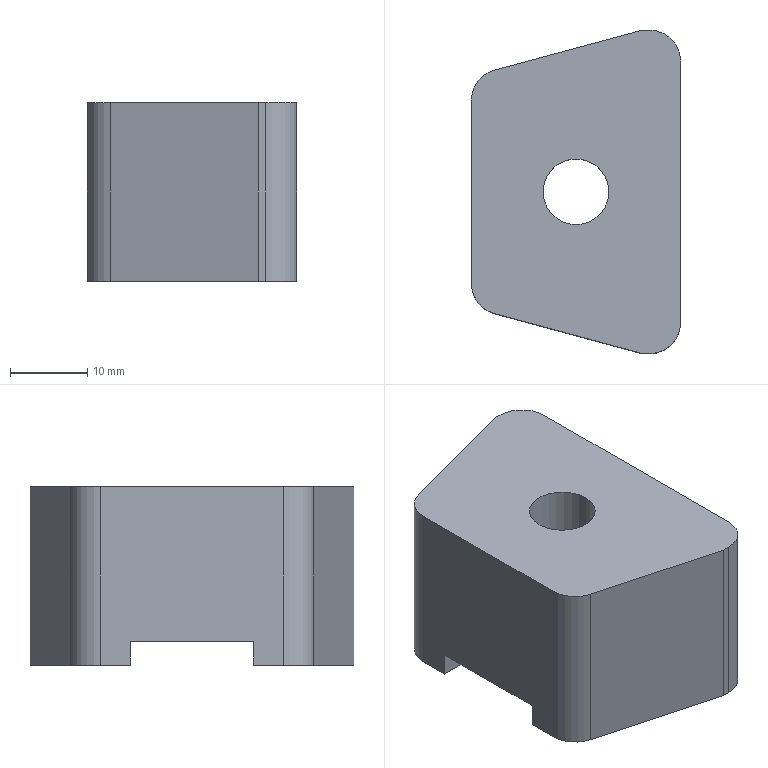Part | NX | features solid 2 | 1 solid | 19 faces | box 27 x 41.761 x 23 mm | volume 19258 mm3 | plane 13 | cylinder 6 | commonest cylinder face diameters 8 x4 8.5 x1 14 x1
STEP:
#1=CARTESIAN_POINT('',(636.324,0.,20.));
#2=VERTEX_POINT('',#1);
#3=CARTESIAN_POINT('',(632.074,0.,20.));
#4=DIRECTION('',(0.,0.,1.));
#5=DIRECTION('',(1.,0.,0.));
#6=AXIS2_PLACEMENT_3D('',#3,#4,#5);
#7=CIRCLE('',#6,4.25);
#8=EDGE_CURVE('',#2,#2,#7,.T.);
#9=ORIENTED_EDGE('',*,*,#8,.F.);
#10=EDGE_LOOP('',(#9));
#11=FACE_BOUND('',#10,.T.);
#12=CARTESIAN_POINT('',(640.659,-20.88,20.));
#13=VERTEX_POINT('',#12);
#14=CARTESIAN_POINT('',(641.574,-20.88,20.));
#15=VERTEX_POINT('',#14);
#16=CARTESIAN_POINT('',(704.285,-20.88,20.));
#17=DIRECTION('',(1.,0.,0.));
#18=VECTOR('',#17,1000.);
#19=LINE('',#16,#18);
#20=EDGE_CURVE('',#13,#15,#19,.T.);
#21=ORIENTED_EDGE('',*,*,#20,.T.);
#22=CARTESIAN_POINT('',(645.574,-16.88,20.));
#23=VERTEX_POINT('',#22);
#24=CARTESIAN_POINT('',(641.574,-16.88,20.));
#25=DIRECTION('',(0.,0.,1.));
#26=DIRECTION('',(1.,0.,0.));
#27=AXIS2_PLACEMENT_3D('',#24,#25,#26);
#28=CIRCLE('',#27,4.);
#29=EDGE_CURVE('',#15,#23,#28,.T.);
#30=ORIENTED_EDGE('',*,*,#29,.T.);
#31=CARTESIAN_POINT('',(645.574,16.88,20.));
#32=VERTEX_POINT('',#31);
#33=CARTESIAN_POINT('',(645.574,-11.19,20.));
#34=DIRECTION('',(0.,-1.,0.));
#35=VECTOR('',#34,1000.);
#36=LINE('',#33,#35);
#37=EDGE_CURVE('',#32,#23,#36,.T.);
#38=ORIENTED_EDGE('',*,*,#37,.F.);
#39=CARTESIAN_POINT('',(641.574,20.88,20.));
#40=VERTEX_POINT('',#39);
#41=CARTESIAN_POINT('',(641.574,16.88,20.));
#42=DIRECTION('',(0.,0.,1.));
#43=DIRECTION('',(1.,0.,0.));
#44=AXIS2_PLACEMENT_3D('',#41,#42,#43);
#45=CIRCLE('',#44,4.);
#46=EDGE_CURVE('',#32,#40,#45,.T.);
#47=ORIENTED_EDGE('',*,*,#46,.T.);
#48=CARTESIAN_POINT('',(640.659,20.88,20.));
#49=VERTEX_POINT('',#48);
#50=CARTESIAN_POINT('',(704.285,20.88,20.));
#51=DIRECTION('',(-1.,0.,0.));
#52=VECTOR('',#51,1000.);
#53=LINE('',#50,#52);
#54=EDGE_CURVE('',#40,#49,#53,.T.);
#55=ORIENTED_EDGE('',*,*,#54,.T.);
#56=CARTESIAN_POINT('',(621.53,15.711,20.));
#57=VERTEX_POINT('',#56);
#58=CARTESIAN_POINT('',(666.85,27.959,20.));
#59=DIRECTION('',(0.9654,0.2609,0.));
#60=VECTOR('',#59,1000.);
#61=LINE('',#58,#60);
#62=EDGE_CURVE('',#49,#57,#61,.F.);
#63=ORIENTED_EDGE('',*,*,#62,.T.);
#64=CARTESIAN_POINT('',(618.574,11.849,20.));
#65=VERTEX_POINT('',#64);
#66=CARTESIAN_POINT('',(622.574,11.849,20.));
#67=DIRECTION('',(0.,0.,1.));
#68=DIRECTION('',(1.,0.,0.));
#69=AXIS2_PLACEMENT_3D('',#66,#67,#68);
#70=CIRCLE('',#69,4.);
#71=EDGE_CURVE('',#57,#65,#70,.T.);
#72=ORIENTED_EDGE('',*,*,#71,.T.);
#73=CARTESIAN_POINT('',(618.574,-11.849,20.));
#74=VERTEX_POINT('',#73);
#75=CARTESIAN_POINT('',(618.574,-7.,20.));
#76=DIRECTION('',(0.,1.,0.));
#77=VECTOR('',#76,1000.);
#78=LINE('',#75,#77);
#79=EDGE_CURVE('',#74,#65,#78,.T.);
#80=ORIENTED_EDGE('',*,*,#79,.F.);
#81=CARTESIAN_POINT('',(621.53,-15.711,20.));
#82=VERTEX_POINT('',#81);
#83=CARTESIAN_POINT('',(622.574,-11.849,20.));
#84=DIRECTION('',(0.,0.,1.));
#85=DIRECTION('',(1.,0.,0.));
#86=AXIS2_PLACEMENT_3D('',#83,#84,#85);
#87=CIRCLE('',#86,4.);
#88=EDGE_CURVE('',#74,#82,#87,.T.);
#89=ORIENTED_EDGE('',*,*,#88,.T.);
#90=CARTESIAN_POINT('',(722.538,-43.01,20.));
#91=DIRECTION('',(-0.9654,0.2609,0.));
#92=VECTOR('',#91,1000.);
#93=LINE('',#90,#92);
#94=EDGE_CURVE('',#82,#13,#93,.F.);
#95=ORIENTED_EDGE('',*,*,#94,.T.);
#96=EDGE_LOOP('',(#21,#30,#38,#47,#55,#63,#72,#80,#89,#95));
#97=FACE_BOUND('',#96,.T.);
#98=CARTESIAN_POINT('',(704.285,-110.548,20.));
#99=DIRECTION('',(0.,0.,1.));
#100=DIRECTION('',(1.,0.,0.));
#101=AXIS2_PLACEMENT_3D('',#98,#99,#100);
#102=PLANE('',#101);
#103=ADVANCED_FACE('',(#11,#97),#102,.T.);
#104=CARTESIAN_POINT('',(645.574,-8.,0.));
#105=VERTEX_POINT('',#104);
#106=CARTESIAN_POINT('',(618.574,-8.,0.));
#107=VERTEX_POINT('',#106);
#108=CARTESIAN_POINT('',(630.85,-8.,0.));
#109=DIRECTION('',(-1.,0.,0.));
#110=VECTOR('',#109,1000.);
#111=LINE('',#108,#110);
#112=EDGE_CURVE('',#105,#107,#111,.T.);
#113=ORIENTED_EDGE('',*,*,#112,.F.);
#114=CARTESIAN_POINT('',(645.574,-8.,-3.));
#115=VERTEX_POINT('',#114);
#116=CARTESIAN_POINT('',(645.574,-8.,-5.));
#117=DIRECTION('',(0.,0.,1.));
#118=VECTOR('',#117,1000.);
#119=LINE('',#116,#118);
#120=EDGE_CURVE('',#115,#105,#119,.T.);
#121=ORIENTED_EDGE('',*,*,#120,.F.);
#122=CARTESIAN_POINT('',(618.574,-8.,-3.));
#123=VERTEX_POINT('',#122);
#124=CARTESIAN_POINT('',(268.879,-8.,-3.));
#125=DIRECTION('',(-1.,0.,0.));
#126=VECTOR('',#125,1000.);
#127=LINE('',#124,#126);
#128=EDGE_CURVE('',#123,#115,#127,.F.);
#129=ORIENTED_EDGE('',*,*,#128,.F.);
#130=CARTESIAN_POINT('',(618.574,-8.,-5.));
#131=DIRECTION('',(0.,0.,1.));
#132=VECTOR('',#131,1000.);
#133=LINE('',#130,#132);
#134=EDGE_CURVE('',#123,#107,#133,.T.);
#135=ORIENTED_EDGE('',*,*,#134,.T.);
#136=EDGE_LOOP('',(#113,#121,#129,#135));
#137=FACE_BOUND('',#136,.T.);
#138=CARTESIAN_POINT('',(630.85,-8.,-5.));
#139=DIRECTION('',(0.,1.,0.));
#140=DIRECTION('',(0.,0.,-1.));
#141=AXIS2_PLACEMENT_3D('',#138,#139,#140);
#142=PLANE('',#141);
#143=ADVANCED_FACE('',(#137),#142,.T.);
#144=CARTESIAN_POINT('',(645.574,-16.88,-3.));
#145=VERTEX_POINT('',#144);
#146=CARTESIAN_POINT('',(645.574,0.,-3.));
#147=DIRECTION('',(0.,1.,0.));
#148=VECTOR('',#147,1000.);
#149=LINE('',#146,#148);
#150=EDGE_CURVE('',#115,#145,#149,.F.);
#151=ORIENTED_EDGE('',*,*,#150,.T.);
#152=CARTESIAN_POINT('',(641.574,-20.88,-3.));
#153=VERTEX_POINT('',#152);
#154=CARTESIAN_POINT('',(641.574,-16.88,-3.));
#155=DIRECTION('',(0.,0.,1.));
#156=DIRECTION('',(1.,0.,0.));
#157=AXIS2_PLACEMENT_3D('',#154,#155,#156);
#158=CIRCLE('',#157,4.);
#159=EDGE_CURVE('',#145,#153,#158,.F.);
#160=ORIENTED_EDGE('',*,*,#159,.T.);
#161=CARTESIAN_POINT('',(640.659,-20.88,-3.));
#162=VERTEX_POINT('',#161);
#163=CARTESIAN_POINT('',(268.879,-20.88,-3.));
#164=DIRECTION('',(1.,0.,0.));
#165=VECTOR('',#164,1000.);
#166=LINE('',#163,#165);
#167=EDGE_CURVE('',#153,#162,#166,.F.);
#168=ORIENTED_EDGE('',*,*,#167,.T.);
#169=CARTESIAN_POINT('',(621.53,-15.711,-3.));
#170=VERTEX_POINT('',#169);
#171=CARTESIAN_POINT('',(637.087,-19.915,-3.));
#172=DIRECTION('',(0.9654,-0.2609,0.));
#173=VECTOR('',#172,1000.);
#174=LINE('',#171,#173);
#175=EDGE_CURVE('',#170,#162,#174,.T.);
#176=ORIENTED_EDGE('',*,*,#175,.F.);
#177=CARTESIAN_POINT('',(618.574,-11.849,-3.));
#178=VERTEX_POINT('',#177);
#179=CARTESIAN_POINT('',(622.574,-11.849,-3.));
#180=DIRECTION('',(0.,0.,1.));
#181=DIRECTION('',(1.,0.,0.));
#182=AXIS2_PLACEMENT_3D('',#179,#180,#181);
#183=CIRCLE('',#182,4.);
#184=EDGE_CURVE('',#170,#178,#183,.F.);
#185=ORIENTED_EDGE('',*,*,#184,.T.);
#186=CARTESIAN_POINT('',(618.574,0.,-3.));
#187=DIRECTION('',(0.,-1.,0.));
#188=VECTOR('',#187,1000.);
#189=LINE('',#186,#188);
#190=EDGE_CURVE('',#178,#123,#189,.F.);
#191=ORIENTED_EDGE('',*,*,#190,.T.);
#192=ORIENTED_EDGE('',*,*,#128,.T.);
#193=EDGE_LOOP('',(#151,#160,#168,#176,#185,#191,#192));
#194=FACE_BOUND('',#193,.T.);
#195=CARTESIAN_POINT('',(268.879,0.,-3.));
#196=DIRECTION('',(0.,0.,1.));
#197=DIRECTION('',(1.,0.,0.));
#198=AXIS2_PLACEMENT_3D('',#195,#196,#197);
#199=PLANE('',#198);
#200=ADVANCED_FACE('',(#194),#199,.F.);
#201=ORIENTED_EDGE('',*,*,#94,.F.);
#202=CARTESIAN_POINT('',(621.53,-15.711,-5.));
#203=DIRECTION('',(0.,0.,-1.));
#204=VECTOR('',#203,1000.);
#205=LINE('',#202,#204);
#206=EDGE_CURVE('',#82,#170,#205,.T.);
#207=ORIENTED_EDGE('',*,*,#206,.T.);
#208=ORIENTED_EDGE('',*,*,#175,.T.);
#209=CARTESIAN_POINT('',(640.659,-20.88,-5.));
#210=DIRECTION('',(0.,0.,-1.));
#211=VECTOR('',#210,1000.);
#212=LINE('',#209,#211);
#213=EDGE_CURVE('',#162,#13,#212,.F.);
#214=ORIENTED_EDGE('',*,*,#213,.T.);
#215=EDGE_LOOP('',(#201,#207,#208,#214));
#216=FACE_BOUND('',#215,.T.);
#217=CARTESIAN_POINT('',(637.087,-19.915,-5.));
#218=DIRECTION('',(0.2609,0.9654,0.));
#219=DIRECTION('',(0.,0.,1.));
#220=AXIS2_PLACEMENT_3D('',#217,#218,#219);
#221=PLANE('',#220);
#222=ADVANCED_FACE('',(#216),#221,.F.);
#223=ORIENTED_EDGE('',*,*,#167,.F.);
#224=CARTESIAN_POINT('',(641.574,-20.88,-5.));
#225=DIRECTION('',(0.,0.,1.));
#226=VECTOR('',#225,1000.);
#227=LINE('',#224,#226);
#228=EDGE_CURVE('',#153,#15,#227,.T.);
#229=ORIENTED_EDGE('',*,*,#228,.T.);
#230=ORIENTED_EDGE('',*,*,#20,.F.);
#231=ORIENTED_EDGE('',*,*,#213,.F.);
#232=EDGE_LOOP('',(#223,#229,#230,#231));
#233=FACE_BOUND('',#232,.T.);
#234=CARTESIAN_POINT('',(630.85,-20.88,-5.));
#235=DIRECTION('',(0.,-1.,0.));
#236=DIRECTION('',(0.,0.,1.));
#237=AXIS2_PLACEMENT_3D('',#234,#235,#236);
#238=PLANE('',#237);
#239=ADVANCED_FACE('',(#233),#238,.T.);
#240=ORIENTED_EDGE('',*,*,#37,.T.);
#241=CARTESIAN_POINT('',(645.574,-16.88,-5.));
#242=DIRECTION('',(0.,0.,1.));
#243=VECTOR('',#242,1000.);
#244=LINE('',#241,#243);
#245=EDGE_CURVE('',#23,#145,#244,.F.);
#246=ORIENTED_EDGE('',*,*,#245,.T.);
#247=ORIENTED_EDGE('',*,*,#150,.F.);
#248=ORIENTED_EDGE('',*,*,#120,.T.);
#249=CARTESIAN_POINT('',(645.574,8.,0.));
#250=VERTEX_POINT('',#249);
#251=CARTESIAN_POINT('',(645.574,1232.968,0.));
#252=DIRECTION('',(0.,-1.,0.));
#253=VECTOR('',#252,1000.);
#254=LINE('',#251,#253);
#255=EDGE_CURVE('',#250,#105,#254,.T.);
#256=ORIENTED_EDGE('',*,*,#255,.F.);
#257=CARTESIAN_POINT('',(645.574,8.,-3.));
#258=VERTEX_POINT('',#257);
#259=CARTESIAN_POINT('',(645.574,8.,-5.));
#260=DIRECTION('',(0.,0.,1.));
#261=VECTOR('',#260,1000.);
#262=LINE('',#259,#261);
#263=EDGE_CURVE('',#258,#250,#262,.T.);
#264=ORIENTED_EDGE('',*,*,#263,.F.);
#265=CARTESIAN_POINT('',(645.574,16.88,-3.));
#266=VERTEX_POINT('',#265);
#267=CARTESIAN_POINT('',(645.574,-11.19,-3.));
#268=DIRECTION('',(0.,-1.,0.));
#269=VECTOR('',#268,1000.);
#270=LINE('',#267,#269);
#271=EDGE_CURVE('',#258,#266,#270,.F.);
#272=ORIENTED_EDGE('',*,*,#271,.T.);
#273=CARTESIAN_POINT('',(645.574,16.88,-5.));
#274=DIRECTION('',(0.,0.,1.));
#275=VECTOR('',#274,1000.);
#276=LINE('',#273,#275);
#277=EDGE_CURVE('',#266,#32,#276,.T.);
#278=ORIENTED_EDGE('',*,*,#277,.T.);
#279=EDGE_LOOP('',(#240,#246,#247,#248,#256,#264,#272,#278));
#280=FACE_BOUND('',#279,.T.);
#281=CARTESIAN_POINT('',(645.574,-11.19,-5.));
#282=DIRECTION('',(1.,0.,0.));
#283=DIRECTION('',(0.,0.,-1.));
#284=AXIS2_PLACEMENT_3D('',#281,#282,#283);
#285=PLANE('',#284);
#286=ADVANCED_FACE('',(#280),#285,.T.);
#287=ORIENTED_EDGE('',*,*,#190,.F.);
#288=CARTESIAN_POINT('',(618.574,-11.849,-5.));
#289=DIRECTION('',(0.,0.,1.));
#290=VECTOR('',#289,1000.);
#291=LINE('',#288,#290);
#292=EDGE_CURVE('',#178,#74,#291,.T.);
#293=ORIENTED_EDGE('',*,*,#292,.T.);
#294=ORIENTED_EDGE('',*,*,#79,.T.);
#295=CARTESIAN_POINT('',(618.574,11.849,-3.));
#296=VERTEX_POINT('',#295);
#297=CARTESIAN_POINT('',(618.574,11.849,-5.));
#298=DIRECTION('',(0.,0.,-1.));
#299=VECTOR('',#298,1000.);
#300=LINE('',#297,#299);
#301=EDGE_CURVE('',#65,#296,#300,.T.);
#302=ORIENTED_EDGE('',*,*,#301,.T.);
#303=CARTESIAN_POINT('',(618.574,8.,-3.));
#304=VERTEX_POINT('',#303);
#305=CARTESIAN_POINT('',(618.574,0.,-3.));
#306=DIRECTION('',(0.,-1.,0.));
#307=VECTOR('',#306,1000.);
#308=LINE('',#305,#307);
#309=EDGE_CURVE('',#304,#296,#308,.F.);
#310=ORIENTED_EDGE('',*,*,#309,.F.);
#311=CARTESIAN_POINT('',(618.574,8.,0.));
#312=VERTEX_POINT('',#311);
#313=CARTESIAN_POINT('',(618.574,8.,-5.));
#314=DIRECTION('',(0.,0.,-1.));
#315=VECTOR('',#314,1000.);
#316=LINE('',#313,#315);
#317=EDGE_CURVE('',#312,#304,#316,.T.);
#318=ORIENTED_EDGE('',*,*,#317,.F.);
#319=CARTESIAN_POINT('',(618.574,1232.968,0.));
#320=DIRECTION('',(0.,1.,0.));
#321=VECTOR('',#320,1000.);
#322=LINE('',#319,#321);
#323=EDGE_CURVE('',#107,#312,#322,.T.);
#324=ORIENTED_EDGE('',*,*,#323,.F.);
#325=ORIENTED_EDGE('',*,*,#134,.F.);
#326=EDGE_LOOP('',(#287,#293,#294,#302,#310,#318,#324,#325));
#327=FACE_BOUND('',#326,.T.);
#328=CARTESIAN_POINT('',(618.574,-7.,-5.));
#329=DIRECTION('',(-1.,0.,0.));
#330=DIRECTION('',(0.,0.,1.));
#331=AXIS2_PLACEMENT_3D('',#328,#329,#330);
#332=PLANE('',#331);
#333=ADVANCED_FACE('',(#327),#332,.T.);
#334=CARTESIAN_POINT('',(630.85,8.,0.));
#335=DIRECTION('',(1.,0.,0.));
#336=VECTOR('',#335,1000.);
#337=LINE('',#334,#336);
#338=EDGE_CURVE('',#312,#250,#337,.T.);
#339=ORIENTED_EDGE('',*,*,#338,.F.);
#340=ORIENTED_EDGE('',*,*,#317,.T.);
#341=CARTESIAN_POINT('',(630.85,8.,-3.));
#342=DIRECTION('',(-1.,0.,0.));
#343=VECTOR('',#342,1000.);
#344=LINE('',#341,#343);
#345=EDGE_CURVE('',#304,#258,#344,.F.);
#346=ORIENTED_EDGE('',*,*,#345,.T.);
#347=ORIENTED_EDGE('',*,*,#263,.T.);
#348=EDGE_LOOP('',(#339,#340,#346,#347));
#349=FACE_BOUND('',#348,.T.);
#350=CARTESIAN_POINT('',(630.85,8.,-5.));
#351=DIRECTION('',(0.,-1.,0.));
#352=DIRECTION('',(0.,0.,-1.));
#353=AXIS2_PLACEMENT_3D('',#350,#351,#352);
#354=PLANE('',#353);
#355=ADVANCED_FACE('',(#349),#354,.T.);
#356=ORIENTED_EDGE('',*,*,#309,.T.);
#357=CARTESIAN_POINT('',(621.53,15.711,-3.));
#358=VERTEX_POINT('',#357);
#359=CARTESIAN_POINT('',(622.574,11.849,-3.));
#360=DIRECTION('',(0.,0.,1.));
#361=DIRECTION('',(1.,0.,0.));
#362=AXIS2_PLACEMENT_3D('',#359,#360,#361);
#363=CIRCLE('',#362,4.);
#364=EDGE_CURVE('',#296,#358,#363,.F.);
#365=ORIENTED_EDGE('',*,*,#364,.T.);
#366=CARTESIAN_POINT('',(640.659,20.88,-3.));
#367=VERTEX_POINT('',#366);
#368=CARTESIAN_POINT('',(288.928,-74.182,-3.));
#369=DIRECTION('',(0.9654,0.2609,0.));
#370=VECTOR('',#369,1000.);
#371=LINE('',#368,#370);
#372=EDGE_CURVE('',#358,#367,#371,.T.);
#373=ORIENTED_EDGE('',*,*,#372,.T.);
#374=CARTESIAN_POINT('',(641.574,20.88,-3.));
#375=VERTEX_POINT('',#374);
#376=CARTESIAN_POINT('',(630.85,20.88,-3.));
#377=DIRECTION('',(1.,0.,0.));
#378=VECTOR('',#377,1000.);
#379=LINE('',#376,#378);
#380=EDGE_CURVE('',#375,#367,#379,.F.);
#381=ORIENTED_EDGE('',*,*,#380,.F.);
#382=CARTESIAN_POINT('',(641.574,16.88,-3.));
#383=DIRECTION('',(0.,0.,1.));
#384=DIRECTION('',(1.,0.,0.));
#385=AXIS2_PLACEMENT_3D('',#382,#383,#384);
#386=CIRCLE('',#385,4.);
#387=EDGE_CURVE('',#375,#266,#386,.F.);
#388=ORIENTED_EDGE('',*,*,#387,.T.);
#389=ORIENTED_EDGE('',*,*,#271,.F.);
#390=ORIENTED_EDGE('',*,*,#345,.F.);
#391=EDGE_LOOP('',(#356,#365,#373,#381,#388,#389,#390));
#392=FACE_BOUND('',#391,.T.);
#393=CARTESIAN_POINT('',(268.879,0.,-3.));
#394=DIRECTION('',(0.,0.,1.));
#395=DIRECTION('',(1.,0.,0.));
#396=AXIS2_PLACEMENT_3D('',#393,#394,#395);
#397=PLANE('',#396);
#398=ADVANCED_FACE('',(#392),#397,.F.);
#399=ORIENTED_EDGE('',*,*,#372,.F.);
#400=CARTESIAN_POINT('',(621.53,15.711,-5.));
#401=DIRECTION('',(0.,0.,1.));
#402=VECTOR('',#401,1000.);
#403=LINE('',#400,#402);
#404=EDGE_CURVE('',#358,#57,#403,.T.);
#405=ORIENTED_EDGE('',*,*,#404,.T.);
#406=ORIENTED_EDGE('',*,*,#62,.F.);
#407=CARTESIAN_POINT('',(640.659,20.88,-5.));
#408=DIRECTION('',(0.,0.,-1.));
#409=VECTOR('',#408,1000.);
#410=LINE('',#407,#409);
#411=EDGE_CURVE('',#367,#49,#410,.F.);
#412=ORIENTED_EDGE('',*,*,#411,.F.);
#413=EDGE_LOOP('',(#399,#405,#406,#412));
#414=FACE_BOUND('',#413,.T.);
#415=CARTESIAN_POINT('',(637.087,19.915,-5.));
#416=DIRECTION('',(0.2609,-0.9654,0.));
#417=DIRECTION('',(0.,0.,1.));
#418=AXIS2_PLACEMENT_3D('',#415,#416,#417);
#419=PLANE('',#418);
#420=ADVANCED_FACE('',(#414),#419,.F.);
#421=ORIENTED_EDGE('',*,*,#54,.F.);
#422=CARTESIAN_POINT('',(641.574,20.88,-5.));
#423=DIRECTION('',(0.,0.,1.));
#424=VECTOR('',#423,1000.);
#425=LINE('',#422,#424);
#426=EDGE_CURVE('',#40,#375,#425,.F.);
#427=ORIENTED_EDGE('',*,*,#426,.T.);
#428=ORIENTED_EDGE('',*,*,#380,.T.);
#429=ORIENTED_EDGE('',*,*,#411,.T.);
#430=EDGE_LOOP('',(#421,#427,#428,#429));
#431=FACE_BOUND('',#430,.T.);
#432=CARTESIAN_POINT('',(630.85,20.88,-5.));
#433=DIRECTION('',(0.,1.,0.));
#434=DIRECTION('',(0.,0.,1.));
#435=AXIS2_PLACEMENT_3D('',#432,#433,#434);
#436=PLANE('',#435);
#437=ADVANCED_FACE('',(#431),#436,.T.);
#438=ORIENTED_EDGE('',*,*,#338,.T.);
#439=ORIENTED_EDGE('',*,*,#255,.T.);
#440=ORIENTED_EDGE('',*,*,#112,.T.);
#441=ORIENTED_EDGE('',*,*,#323,.T.);
#442=EDGE_LOOP('',(#438,#439,#440,#441));
#443=FACE_BOUND('',#442,.T.);
#444=CARTESIAN_POINT('',(625.074,0.,0.));
#445=VERTEX_POINT('',#444);
#446=CARTESIAN_POINT('',(632.074,0.,0.));
#447=DIRECTION('',(0.,0.,-1.));
#448=DIRECTION('',(-1.,0.,0.));
#449=AXIS2_PLACEMENT_3D('',#446,#447,#448);
#450=CIRCLE('',#449,7.);
#451=EDGE_CURVE('',#445,#445,#450,.F.);
#452=ORIENTED_EDGE('',*,*,#451,.T.);
#453=EDGE_LOOP('',(#452));
#454=FACE_BOUND('',#453,.T.);
#455=CARTESIAN_POINT('',(-316.443,1232.968,0.));
#456=DIRECTION('',(0.,0.,-1.));
#457=DIRECTION('',(-0.9659,0.2588,0.));
#458=AXIS2_PLACEMENT_3D('',#455,#456,#457);
#459=PLANE('',#458);
#460=ADVANCED_FACE('',(#443,#454),#459,.T.);
#461=ORIENTED_EDGE('',*,*,#159,.F.);
#462=ORIENTED_EDGE('',*,*,#245,.F.);
#463=ORIENTED_EDGE('',*,*,#29,.F.);
#464=ORIENTED_EDGE('',*,*,#228,.F.);
#465=EDGE_LOOP('',(#461,#462,#463,#464));
#466=FACE_BOUND('',#465,.T.);
#467=CARTESIAN_POINT('',(641.574,-16.88,-5.));
#468=DIRECTION('',(0.,0.,1.));
#469=DIRECTION('',(1.,0.,0.));
#470=AXIS2_PLACEMENT_3D('',#467,#468,#469);
#471=CYLINDRICAL_SURFACE('',#470,4.);
#472=ADVANCED_FACE('',(#466),#471,.T.);
#473=ORIENTED_EDGE('',*,*,#88,.F.);
#474=ORIENTED_EDGE('',*,*,#292,.F.);
#475=ORIENTED_EDGE('',*,*,#184,.F.);
#476=ORIENTED_EDGE('',*,*,#206,.F.);
#477=EDGE_LOOP('',(#473,#474,#475,#476));
#478=FACE_BOUND('',#477,.T.);
#479=CARTESIAN_POINT('',(622.574,-11.849,-5.));
#480=DIRECTION('',(0.,0.,1.));
#481=DIRECTION('',(1.,0.,0.));
#482=AXIS2_PLACEMENT_3D('',#479,#480,#481);
#483=CYLINDRICAL_SURFACE('',#482,4.);
#484=ADVANCED_FACE('',(#478),#483,.T.);
#485=ORIENTED_EDGE('',*,*,#364,.F.);
#486=ORIENTED_EDGE('',*,*,#301,.F.);
#487=ORIENTED_EDGE('',*,*,#71,.F.);
#488=ORIENTED_EDGE('',*,*,#404,.F.);
#489=EDGE_LOOP('',(#485,#486,#487,#488));
#490=FACE_BOUND('',#489,.T.);
#491=CARTESIAN_POINT('',(622.574,11.849,-5.));
#492=DIRECTION('',(0.,0.,-1.));
#493=DIRECTION('',(-1.,0.,0.));
#494=AXIS2_PLACEMENT_3D('',#491,#492,#493);
#495=CYLINDRICAL_SURFACE('',#494,4.);
#496=ADVANCED_FACE('',(#490),#495,.T.);
#497=ORIENTED_EDGE('',*,*,#387,.F.);
#498=ORIENTED_EDGE('',*,*,#426,.F.);
#499=ORIENTED_EDGE('',*,*,#46,.F.);
#500=ORIENTED_EDGE('',*,*,#277,.F.);
#501=EDGE_LOOP('',(#497,#498,#499,#500));
#502=FACE_BOUND('',#501,.T.);
#503=CARTESIAN_POINT('',(641.574,16.88,-5.));
#504=DIRECTION('',(0.,0.,1.));
#505=DIRECTION('',(1.,0.,0.));
#506=AXIS2_PLACEMENT_3D('',#503,#504,#505);
#507=CYLINDRICAL_SURFACE('',#506,4.);
#508=ADVANCED_FACE('',(#502),#507,.T.);
#509=ORIENTED_EDGE('',*,*,#8,.T.);
#510=EDGE_LOOP('',(#509));
#511=FACE_BOUND('',#510,.T.);
#512=CARTESIAN_POINT('',(636.324,0.,10.));
#513=VERTEX_POINT('',#512);
#514=CARTESIAN_POINT('',(632.074,0.,10.));
#515=DIRECTION('',(0.,0.,1.));
#516=DIRECTION('',(1.,0.,0.));
#517=AXIS2_PLACEMENT_3D('',#514,#515,#516);
#518=CIRCLE('',#517,4.25);
#519=EDGE_CURVE('',#513,#513,#518,.F.);
#520=ORIENTED_EDGE('',*,*,#519,.T.);
#521=EDGE_LOOP('',(#520));
#522=FACE_BOUND('',#521,.T.);
#523=CARTESIAN_POINT('',(632.074,0.,50.));
#524=DIRECTION('',(0.,0.,1.));
#525=DIRECTION('',(1.,0.,0.));
#526=AXIS2_PLACEMENT_3D('',#523,#524,#525);
#527=CYLINDRICAL_SURFACE('',#526,4.25);
#528=ADVANCED_FACE('',(#511,#522),#527,.F.);
#529=ORIENTED_EDGE('',*,*,#519,.F.);
#530=EDGE_LOOP('',(#529));
#531=FACE_BOUND('',#530,.T.);
#532=CARTESIAN_POINT('',(639.074,0.,10.));
#533=VERTEX_POINT('',#532);
#534=CARTESIAN_POINT('',(632.074,0.,10.));
#535=DIRECTION('',(0.,0.,1.));
#536=DIRECTION('',(1.,0.,0.));
#537=AXIS2_PLACEMENT_3D('',#534,#535,#536);
#538=CIRCLE('',#537,7.);
#539=EDGE_CURVE('',#533,#533,#538,.F.);
#540=ORIENTED_EDGE('',*,*,#539,.T.);
#541=EDGE_LOOP('',(#540));
#542=FACE_BOUND('',#541,.T.);
#543=CARTESIAN_POINT('',(632.074,0.,10.));
#544=DIRECTION('',(0.,0.,1.));
#545=DIRECTION('',(1.,0.,0.));
#546=AXIS2_PLACEMENT_3D('',#543,#544,#545);
#547=PLANE('',#546);
#548=ADVANCED_FACE('',(#531,#542),#547,.F.);
#549=ORIENTED_EDGE('',*,*,#539,.F.);
#550=EDGE_LOOP('',(#549));
#551=FACE_BOUND('',#550,.T.);
#552=ORIENTED_EDGE('',*,*,#451,.F.);
#553=EDGE_LOOP('',(#552));
#554=FACE_BOUND('',#553,.T.);
#555=CARTESIAN_POINT('',(632.074,0.,0.));
#556=DIRECTION('',(0.,0.,1.));
#557=DIRECTION('',(1.,0.,0.));
#558=AXIS2_PLACEMENT_3D('',#555,#556,#557);
#559=CYLINDRICAL_SURFACE('',#558,7.);
#560=ADVANCED_FACE('',(#551,#554),#559,.F.);
#561=CLOSED_SHELL('',(#103,#143,#200,#222,#239,#286,#333,#355,#398,#420,#437,#460,#472,#484,#496,#508,#528,#548,#560));
#562=MANIFOLD_SOLID_BREP('',#561);
#563=(LENGTH_UNIT()NAMED_UNIT(*)SI_UNIT(.MILLI.,.METRE.));
#564=UNCERTAINTY_MEASURE_WITH_UNIT(LENGTH_MEASURE(0.00001),#563,'','');
#565=(NAMED_UNIT(*)PLANE_ANGLE_UNIT()SI_UNIT($,.RADIAN.));
#566=(NAMED_UNIT(*)SI_UNIT($,.STERADIAN.)SOLID_ANGLE_UNIT());
#567=(GEOMETRIC_REPRESENTATION_CONTEXT(3)GLOBAL_UNCERTAINTY_ASSIGNED_CONTEXT((#564))GLOBAL_UNIT_ASSIGNED_CONTEXT((#563,#565,#566))REPRESENTATION_CONTEXT('',''));
#568=ADVANCED_BREP_SHAPE_REPRESENTATION('',(#562),#567);